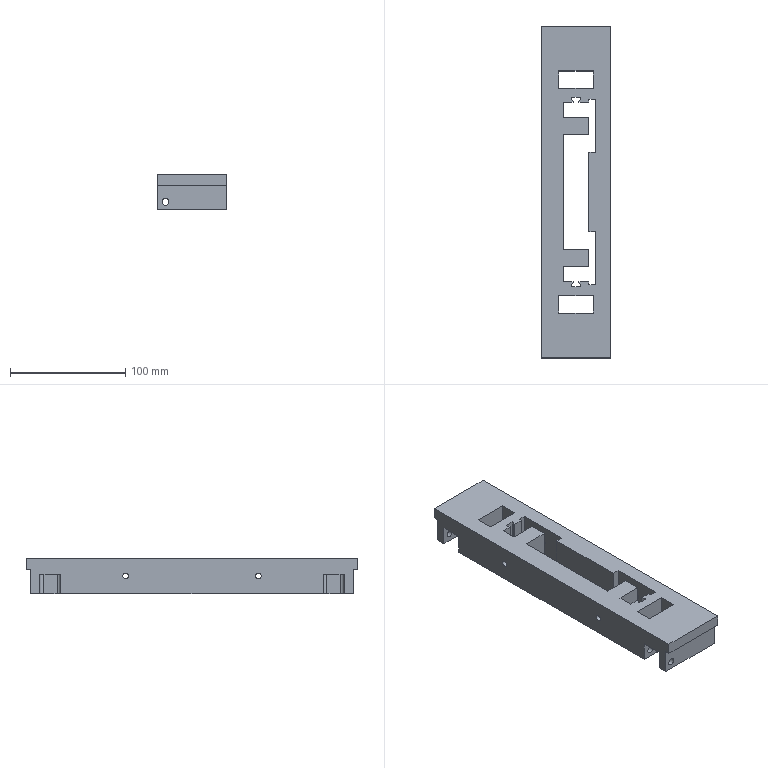Part | STEP file | 1 solid | 81 faces | box 60 x 288 x 31.2 mm | volume 374640 mm3 | plane 54 | cylinder 23 | cone 4 | commonest cylinder face diameters 0.52 x4 1.08 x4 4.2 x4 5.01 x4 6 x4 6.02 x3